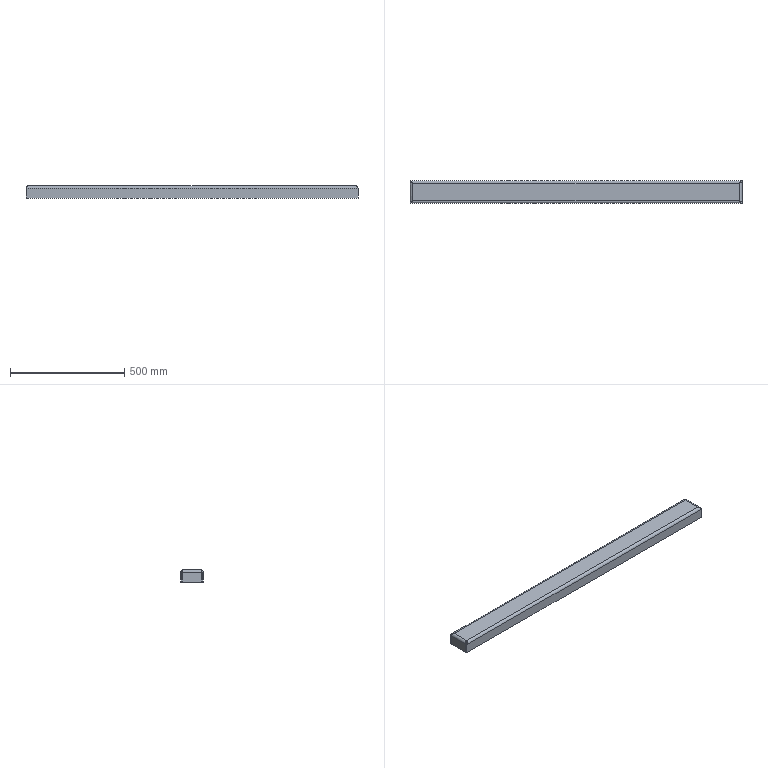Part | STEP file | VD-SYL0380DJ1006_1_1_1-2-492428 | 1 solid | 38 faces | box 1450 x 100 x 54 mm | volume 1690826 mm3 | plane 22 | spline 8 | cylinder 8 | commonest cylinder face diameters 10 x4 22 x4